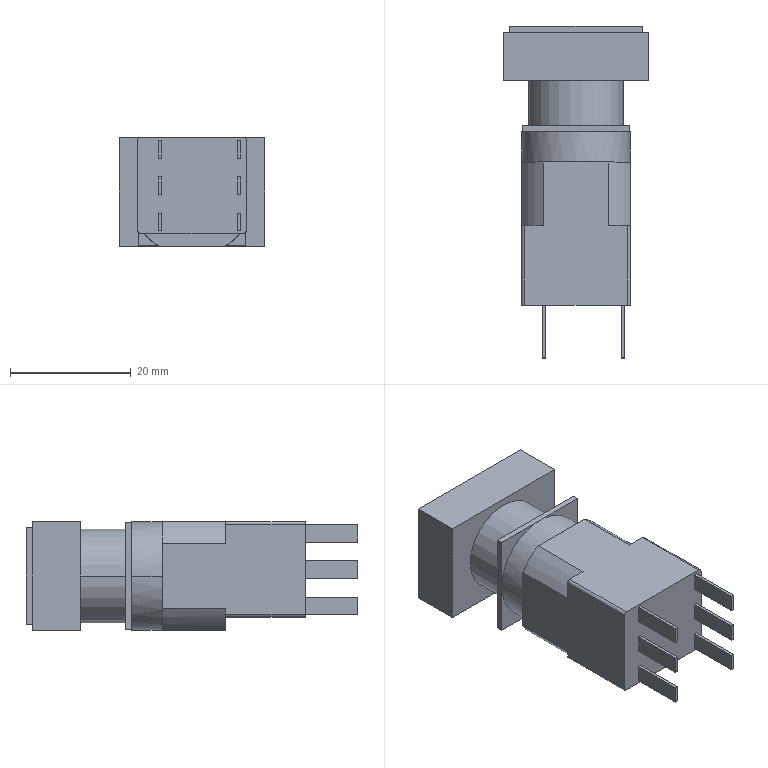Part | NX | 1 solid | 78 faces | box 24 x 54.9 x 18 mm | volume 13819 mm3 | plane 66 | cylinder 12 | commonest cylinder face diameters 1 x4 21 x4 15.6 x2 17.9 x2